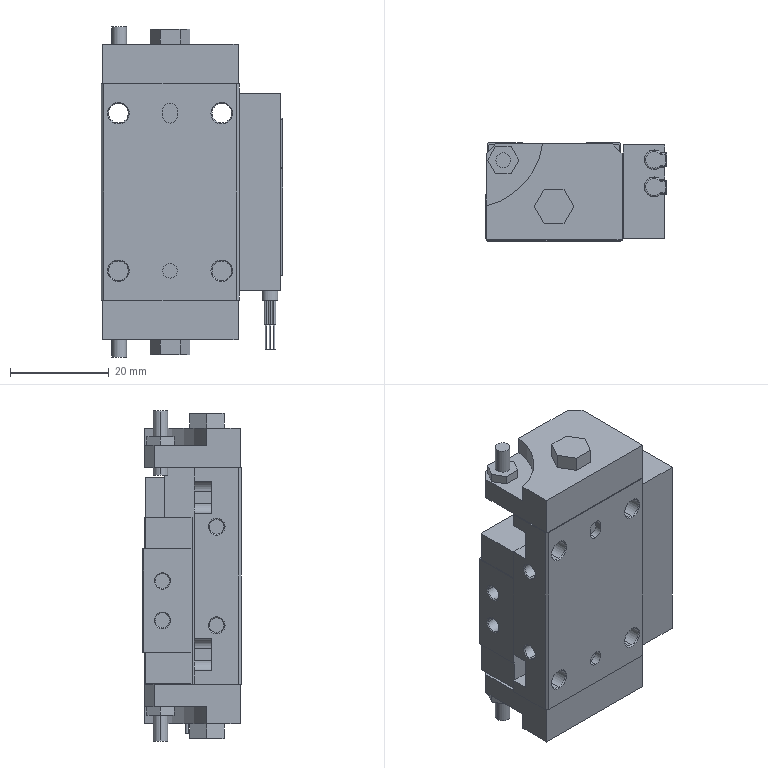Part | NX | 4 solids | 365 faces | box 36.91 x 20 x 67 mm | volume 34044 mm3 | plane 195 | cylinder 112 | cone 48 | torus 6 | spline 4 | commonest cylinder face diameters 3 x38 4 x26 0.5 x12 0.75 x12 2.05 x8 0.6 x6